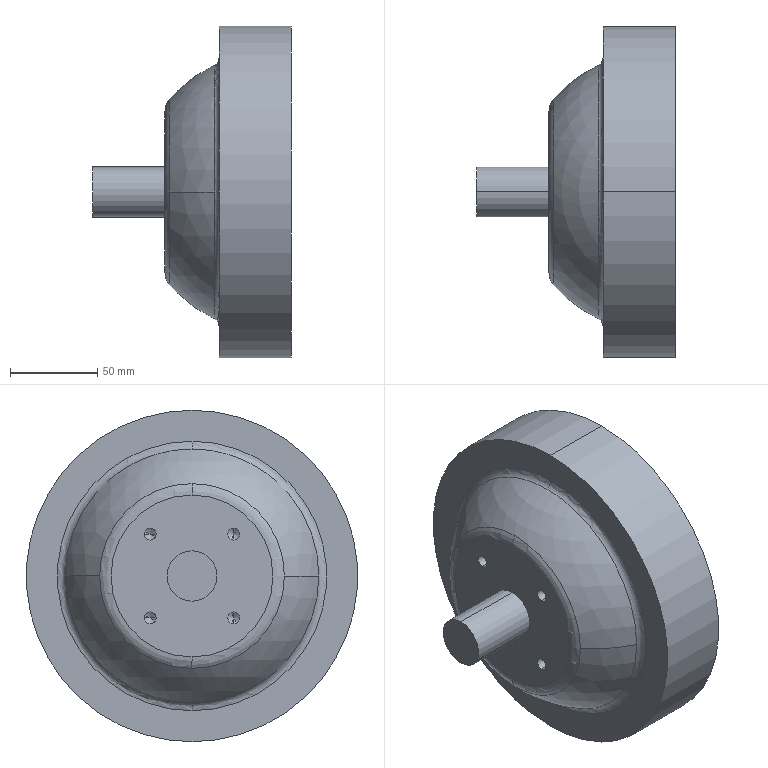Part | NX | features BREP 1 | 1 solid | 30 faces | box 114 x 190 x 190 mm | volume 1604284 mm3 | cylinder 12 | cone 8 | plane 4 | torus 4 | sphere 2 | commonest cylinder face diameters 6.8 x8 28.848 x2 190 x2
STEP:
#1=CARTESIAN_POINT('',(-72.5,0.,-46.402));
#2=VERTEX_POINT('',#1);
#3=CARTESIAN_POINT('',(-72.5,0.,46.402));
#4=VERTEX_POINT('',#3);
#5=CARTESIAN_POINT('',(-72.5,0.,0.));
#6=DIRECTION('',(-1.,0.,0.));
#7=DIRECTION('',(0.,0.,-1.));
#8=AXIS2_PLACEMENT_3D('',#5,#6,#7);
#9=CIRCLE('',#8,46.402);
#10=EDGE_CURVE('',#2,#4,#9,.T.);
#11=ORIENTED_EDGE('',*,*,#10,.T.);
#12=CARTESIAN_POINT('',(-72.5,0.,0.));
#13=DIRECTION('',(-1.,0.,0.));
#14=DIRECTION('',(0.,0.,1.));
#15=AXIS2_PLACEMENT_3D('',#12,#13,#14);
#16=CIRCLE('',#15,46.402);
#17=EDGE_CURVE('',#4,#2,#16,.T.);
#18=ORIENTED_EDGE('',*,*,#17,.T.);
#19=EDGE_LOOP('',(#11,#18));
#20=FACE_BOUND('',#19,.T.);
#21=CARTESIAN_POINT('',(-72.5,0.,14.424));
#22=VERTEX_POINT('',#21);
#23=CARTESIAN_POINT('',(-72.5,0.,-14.424));
#24=VERTEX_POINT('',#23);
#25=CARTESIAN_POINT('',(-72.5,0.,0.));
#26=DIRECTION('',(1.,0.,0.));
#27=DIRECTION('',(0.,0.,1.));
#28=AXIS2_PLACEMENT_3D('',#25,#26,#27);
#29=CIRCLE('',#28,14.424);
#30=EDGE_CURVE('',#22,#24,#29,.T.);
#31=ORIENTED_EDGE('',*,*,#30,.T.);
#32=CARTESIAN_POINT('',(-72.5,0.,0.));
#33=DIRECTION('',(1.,0.,0.));
#34=DIRECTION('',(0.,0.,-1.));
#35=AXIS2_PLACEMENT_3D('',#32,#33,#34);
#36=CIRCLE('',#35,14.424);
#37=EDGE_CURVE('',#24,#22,#36,.T.);
#38=ORIENTED_EDGE('',*,*,#37,.T.);
#39=EDGE_LOOP('',(#31,#38));
#40=FACE_BOUND('',#39,.T.);
#41=CARTESIAN_POINT('',(-72.5,24.,-27.4));
#42=VERTEX_POINT('',#41);
#43=CARTESIAN_POINT('',(-72.5,24.,-20.6));
#44=VERTEX_POINT('',#43);
#45=CARTESIAN_POINT('',(-72.5,24.,-24.));
#46=DIRECTION('',(1.,0.,0.));
#47=DIRECTION('',(0.,0.,-1.));
#48=AXIS2_PLACEMENT_3D('',#45,#46,#47);
#49=CIRCLE('',#48,3.4);
#50=EDGE_CURVE('',#42,#44,#49,.T.);
#51=ORIENTED_EDGE('',*,*,#50,.T.);
#52=CARTESIAN_POINT('',(-72.5,24.,-24.));
#53=DIRECTION('',(1.,0.,0.));
#54=DIRECTION('',(0.,0.,1.));
#55=AXIS2_PLACEMENT_3D('',#52,#53,#54);
#56=CIRCLE('',#55,3.4);
#57=EDGE_CURVE('',#44,#42,#56,.T.);
#58=ORIENTED_EDGE('',*,*,#57,.T.);
#59=EDGE_LOOP('',(#51,#58));
#60=FACE_BOUND('',#59,.T.);
#61=CARTESIAN_POINT('',(-72.5,24.,20.6));
#62=VERTEX_POINT('',#61);
#63=CARTESIAN_POINT('',(-72.5,24.,27.4));
#64=VERTEX_POINT('',#63);
#65=CARTESIAN_POINT('',(-72.5,24.,24.));
#66=DIRECTION('',(1.,0.,0.));
#67=DIRECTION('',(0.,0.,-1.));
#68=AXIS2_PLACEMENT_3D('',#65,#66,#67);
#69=CIRCLE('',#68,3.4);
#70=EDGE_CURVE('',#62,#64,#69,.T.);
#71=ORIENTED_EDGE('',*,*,#70,.T.);
#72=CARTESIAN_POINT('',(-72.5,24.,24.));
#73=DIRECTION('',(1.,0.,0.));
#74=DIRECTION('',(0.,0.,1.));
#75=AXIS2_PLACEMENT_3D('',#72,#73,#74);
#76=CIRCLE('',#75,3.4);
#77=EDGE_CURVE('',#64,#62,#76,.T.);
#78=ORIENTED_EDGE('',*,*,#77,.T.);
#79=EDGE_LOOP('',(#71,#78));
#80=FACE_BOUND('',#79,.T.);
#81=CARTESIAN_POINT('',(-72.5,-24.,20.6));
#82=VERTEX_POINT('',#81);
#83=CARTESIAN_POINT('',(-72.5,-24.,27.4));
#84=VERTEX_POINT('',#83);
#85=CARTESIAN_POINT('',(-72.5,-24.,24.));
#86=DIRECTION('',(1.,0.,0.));
#87=DIRECTION('',(0.,0.,-1.));
#88=AXIS2_PLACEMENT_3D('',#85,#86,#87);
#89=CIRCLE('',#88,3.4);
#90=EDGE_CURVE('',#82,#84,#89,.T.);
#91=ORIENTED_EDGE('',*,*,#90,.T.);
#92=CARTESIAN_POINT('',(-72.5,-24.,24.));
#93=DIRECTION('',(1.,0.,0.));
#94=DIRECTION('',(0.,0.,1.));
#95=AXIS2_PLACEMENT_3D('',#92,#93,#94);
#96=CIRCLE('',#95,3.4);
#97=EDGE_CURVE('',#84,#82,#96,.T.);
#98=ORIENTED_EDGE('',*,*,#97,.T.);
#99=EDGE_LOOP('',(#91,#98));
#100=FACE_BOUND('',#99,.T.);
#101=CARTESIAN_POINT('',(-72.5,-24.,-27.4));
#102=VERTEX_POINT('',#101);
#103=CARTESIAN_POINT('',(-72.5,-24.,-20.6));
#104=VERTEX_POINT('',#103);
#105=CARTESIAN_POINT('',(-72.5,-24.,-24.));
#106=DIRECTION('',(1.,0.,0.));
#107=DIRECTION('',(0.,0.,-1.));
#108=AXIS2_PLACEMENT_3D('',#105,#106,#107);
#109=CIRCLE('',#108,3.4);
#110=EDGE_CURVE('',#102,#104,#109,.T.);
#111=ORIENTED_EDGE('',*,*,#110,.T.);
#112=CARTESIAN_POINT('',(-72.5,-24.,-24.));
#113=DIRECTION('',(1.,0.,0.));
#114=DIRECTION('',(0.,0.,1.));
#115=AXIS2_PLACEMENT_3D('',#112,#113,#114);
#116=CIRCLE('',#115,3.4);
#117=EDGE_CURVE('',#104,#102,#116,.T.);
#118=ORIENTED_EDGE('',*,*,#117,.T.);
#119=EDGE_LOOP('',(#111,#118));
#120=FACE_BOUND('',#119,.T.);
#121=CARTESIAN_POINT('',(-72.5,-48.837,-48.837));
#122=DIRECTION('',(-1.,0.,0.));
#123=DIRECTION('',(0.,0.,1.));
#124=AXIS2_PLACEMENT_3D('',#121,#122,#123);
#125=PLANE('',#124);
#126=ADVANCED_FACE('',(#20,#40,#60,#80,#100,#120),#125,.T.);
#127=CARTESIAN_POINT('',(-70.048,0.,-52.961));
#128=VERTEX_POINT('',#127);
#129=CARTESIAN_POINT('',(-70.048,52.961,0.));
#130=VERTEX_POINT('',#129);
#131=CARTESIAN_POINT('',(-70.048,0.,0.));
#132=DIRECTION('',(1.,0.,0.));
#133=DIRECTION('',(0.,0.,-1.));
#134=AXIS2_PLACEMENT_3D('',#131,#132,#133);
#135=CIRCLE('',#134,52.961);
#136=EDGE_CURVE('',#128,#130,#135,.T.);
#137=ORIENTED_EDGE('',*,*,#136,.F.);
#138=CARTESIAN_POINT('',(-62.5,0.,-46.402));
#139=DIRECTION('',(0.,-1.,0.));
#140=DIRECTION('',(-1.,0.,0.));
#141=AXIS2_PLACEMENT_3D('',#138,#139,#140);
#142=CIRCLE('',#141,10.);
#143=EDGE_CURVE('',#2,#128,#142,.T.);
#144=ORIENTED_EDGE('',*,*,#143,.F.);
#145=ORIENTED_EDGE('',*,*,#17,.F.);
#146=CARTESIAN_POINT('',(-70.048,0.,52.961));
#147=VERTEX_POINT('',#146);
#148=CARTESIAN_POINT('',(-62.5,0.,46.402));
#149=DIRECTION('',(0.,1.,0.));
#150=DIRECTION('',(-1.,0.,0.));
#151=AXIS2_PLACEMENT_3D('',#148,#149,#150);
#152=CIRCLE('',#151,10.);
#153=EDGE_CURVE('',#4,#147,#152,.T.);
#154=ORIENTED_EDGE('',*,*,#153,.T.);
#155=CARTESIAN_POINT('',(-70.048,0.,0.));
#156=DIRECTION('',(1.,0.,0.));
#157=DIRECTION('',(0.,1.,0.));
#158=AXIS2_PLACEMENT_3D('',#155,#156,#157);
#159=CIRCLE('',#158,52.961);
#160=EDGE_CURVE('',#130,#147,#159,.T.);
#161=ORIENTED_EDGE('',*,*,#160,.F.);
#162=EDGE_LOOP('',(#137,#144,#145,#154,#161));
#163=FACE_BOUND('',#162,.T.);
#164=CARTESIAN_POINT('',(-62.5,0.,0.));
#165=DIRECTION('',(-1.,0.,0.));
#166=DIRECTION('',(0.,0.,1.));
#167=AXIS2_PLACEMENT_3D('',#164,#165,#166);
#168=TOROIDAL_SURFACE('',#167,46.402,10.);
#169=ADVANCED_FACE('',(#163),#168,.T.);
#170=CARTESIAN_POINT('',(-44.225,-72.702,0.));
#171=VERTEX_POINT('',#170);
#172=CARTESIAN_POINT('',(-70.048,-52.961,0.));
#173=VERTEX_POINT('',#172);
#174=CARTESIAN_POINT('',(-9.104,0.,0.));
#175=DIRECTION('',(0.,0.,-1.));
#176=DIRECTION('',(-0.435,-0.9004,0.));
#177=AXIS2_PLACEMENT_3D('',#174,#175,#176);
#178=CIRCLE('',#177,80.74);
#179=EDGE_CURVE('',#171,#173,#178,.T.);
#180=ORIENTED_EDGE('',*,*,#179,.F.);
#181=CARTESIAN_POINT('',(-44.225,0.,72.702));
#182=VERTEX_POINT('',#181);
#183=CARTESIAN_POINT('',(-44.225,0.,0.));
#184=DIRECTION('',(-1.,0.,0.));
#185=DIRECTION('',(0.,-1.,0.));
#186=AXIS2_PLACEMENT_3D('',#183,#184,#185);
#187=CIRCLE('',#186,72.702);
#188=EDGE_CURVE('',#171,#182,#187,.T.);
#189=ORIENTED_EDGE('',*,*,#188,.T.);
#190=CARTESIAN_POINT('',(-44.225,72.702,0.));
#191=VERTEX_POINT('',#190);
#192=CARTESIAN_POINT('',(-44.225,0.,0.));
#193=DIRECTION('',(-1.,0.,0.));
#194=DIRECTION('',(0.,0.,1.));
#195=AXIS2_PLACEMENT_3D('',#192,#193,#194);
#196=CIRCLE('',#195,72.702);
#197=EDGE_CURVE('',#182,#191,#196,.T.);
#198=ORIENTED_EDGE('',*,*,#197,.T.);
#199=CARTESIAN_POINT('',(-9.104,0.,0.));
#200=DIRECTION('',(0.,0.,1.));
#201=DIRECTION('',(-0.435,0.9004,0.));
#202=AXIS2_PLACEMENT_3D('',#199,#200,#201);
#203=CIRCLE('',#202,80.74);
#204=EDGE_CURVE('',#191,#130,#203,.T.);
#205=ORIENTED_EDGE('',*,*,#204,.T.);
#206=ORIENTED_EDGE('',*,*,#160,.T.);
#207=CARTESIAN_POINT('',(-70.048,0.,0.));
#208=DIRECTION('',(1.,0.,0.));
#209=DIRECTION('',(0.,0.,1.));
#210=AXIS2_PLACEMENT_3D('',#207,#208,#209);
#211=CIRCLE('',#210,52.961);
#212=EDGE_CURVE('',#147,#173,#211,.T.);
#213=ORIENTED_EDGE('',*,*,#212,.T.);
#214=EDGE_LOOP('',(#180,#189,#198,#205,#206,#213));
#215=FACE_BOUND('',#214,.T.);
#216=CARTESIAN_POINT('',(-9.104,0.,0.));
#217=DIRECTION('',(0.,0.,1.));
#218=DIRECTION('',(0.,1.,0.));
#219=AXIS2_PLACEMENT_3D('',#216,#217,#218);
#220=SPHERICAL_SURFACE('',#219,80.74);
#221=ADVANCED_FACE('',(#215),#220,.T.);
#222=CARTESIAN_POINT('',(-70.048,0.,0.));
#223=DIRECTION('',(1.,0.,0.));
#224=DIRECTION('',(0.,-1.,0.));
#225=AXIS2_PLACEMENT_3D('',#222,#223,#224);
#226=CIRCLE('',#225,52.961);
#227=EDGE_CURVE('',#173,#128,#226,.T.);
#228=ORIENTED_EDGE('',*,*,#227,.F.);
#229=ORIENTED_EDGE('',*,*,#212,.F.);
#230=ORIENTED_EDGE('',*,*,#153,.F.);
#231=ORIENTED_EDGE('',*,*,#10,.F.);
#232=ORIENTED_EDGE('',*,*,#143,.T.);
#233=EDGE_LOOP('',(#228,#229,#230,#231,#232));
#234=FACE_BOUND('',#233,.T.);
#235=CARTESIAN_POINT('',(-62.5,0.,0.));
#236=DIRECTION('',(-1.,0.,0.));
#237=DIRECTION('',(0.,0.,-1.));
#238=AXIS2_PLACEMENT_3D('',#235,#236,#237);
#239=TOROIDAL_SURFACE('',#238,46.402,10.);
#240=ADVANCED_FACE('',(#234),#239,.T.);
#241=ORIENTED_EDGE('',*,*,#227,.T.);
#242=ORIENTED_EDGE('',*,*,#136,.T.);
#243=ORIENTED_EDGE('',*,*,#204,.F.);
#244=CARTESIAN_POINT('',(-44.225,0.,-72.702));
#245=VERTEX_POINT('',#244);
#246=CARTESIAN_POINT('',(-44.225,0.,0.));
#247=DIRECTION('',(-1.,0.,0.));
#248=DIRECTION('',(0.,1.,0.));
#249=AXIS2_PLACEMENT_3D('',#246,#247,#248);
#250=CIRCLE('',#249,72.702);
#251=EDGE_CURVE('',#191,#245,#250,.T.);
#252=ORIENTED_EDGE('',*,*,#251,.T.);
#253=CARTESIAN_POINT('',(-44.225,0.,0.));
#254=DIRECTION('',(-1.,0.,0.));
#255=DIRECTION('',(0.,0.,-1.));
#256=AXIS2_PLACEMENT_3D('',#253,#254,#255);
#257=CIRCLE('',#256,72.702);
#258=EDGE_CURVE('',#245,#171,#257,.T.);
#259=ORIENTED_EDGE('',*,*,#258,.T.);
#260=ORIENTED_EDGE('',*,*,#179,.T.);
#261=EDGE_LOOP('',(#241,#242,#243,#252,#259,#260));
#262=FACE_BOUND('',#261,.T.);
#263=CARTESIAN_POINT('',(-9.104,0.,0.));
#264=DIRECTION('',(0.,0.,-1.));
#265=DIRECTION('',(0.,-1.,0.));
#266=AXIS2_PLACEMENT_3D('',#263,#264,#265);
#267=SPHERICAL_SURFACE('',#266,80.74);
#268=ADVANCED_FACE('',(#262),#267,.T.);
#269=CARTESIAN_POINT('',(-41.4,0.,-77.204));
#270=VERTEX_POINT('',#269);
#271=CARTESIAN_POINT('',(-46.4,0.,-77.204));
#272=DIRECTION('',(0.,-1.,0.));
#273=DIRECTION('',(1.,0.,0.));
#274=AXIS2_PLACEMENT_3D('',#271,#272,#273);
#275=CIRCLE('',#274,5.);
#276=EDGE_CURVE('',#270,#245,#275,.T.);
#277=ORIENTED_EDGE('',*,*,#276,.F.);
#278=CARTESIAN_POINT('',(-41.4,0.,77.204));
#279=VERTEX_POINT('',#278);
#280=CARTESIAN_POINT('',(-41.4,0.,0.));
#281=DIRECTION('',(1.,0.,0.));
#282=DIRECTION('',(0.,0.,1.));
#283=AXIS2_PLACEMENT_3D('',#280,#281,#282);
#284=CIRCLE('',#283,77.204);
#285=EDGE_CURVE('',#279,#270,#284,.T.);
#286=ORIENTED_EDGE('',*,*,#285,.F.);
#287=CARTESIAN_POINT('',(-46.4,0.,77.204));
#288=DIRECTION('',(0.,1.,0.));
#289=DIRECTION('',(1.,0.,0.));
#290=AXIS2_PLACEMENT_3D('',#287,#288,#289);
#291=CIRCLE('',#290,5.);
#292=EDGE_CURVE('',#279,#182,#291,.T.);
#293=ORIENTED_EDGE('',*,*,#292,.T.);
#294=ORIENTED_EDGE('',*,*,#188,.F.);
#295=ORIENTED_EDGE('',*,*,#258,.F.);
#296=EDGE_LOOP('',(#277,#286,#293,#294,#295));
#297=FACE_BOUND('',#296,.T.);
#298=CARTESIAN_POINT('',(-46.4,0.,0.));
#299=DIRECTION('',(1.,0.,0.));
#300=DIRECTION('',(0.,0.,-1.));
#301=AXIS2_PLACEMENT_3D('',#298,#299,#300);
#302=TOROIDAL_SURFACE('',#301,77.204,5.);
#303=ADVANCED_FACE('',(#297),#302,.F.);
#304=ORIENTED_EDGE('',*,*,#251,.F.);
#305=ORIENTED_EDGE('',*,*,#197,.F.);
#306=ORIENTED_EDGE('',*,*,#292,.F.);
#307=CARTESIAN_POINT('',(-41.4,0.,0.));
#308=DIRECTION('',(1.,0.,0.));
#309=DIRECTION('',(0.,0.,-1.));
#310=AXIS2_PLACEMENT_3D('',#307,#308,#309);
#311=CIRCLE('',#310,77.204);
#312=EDGE_CURVE('',#270,#279,#311,.T.);
#313=ORIENTED_EDGE('',*,*,#312,.F.);
#314=ORIENTED_EDGE('',*,*,#276,.T.);
#315=EDGE_LOOP('',(#304,#305,#306,#313,#314));
#316=FACE_BOUND('',#315,.T.);
#317=CARTESIAN_POINT('',(-46.4,0.,0.));
#318=DIRECTION('',(1.,0.,0.));
#319=DIRECTION('',(0.,0.,1.));
#320=AXIS2_PLACEMENT_3D('',#317,#318,#319);
#321=TOROIDAL_SURFACE('',#320,77.204,5.);
#322=ADVANCED_FACE('',(#316),#321,.F.);
#323=CARTESIAN_POINT('',(-41.4,0.,95.));
#324=VERTEX_POINT('',#323);
#325=CARTESIAN_POINT('',(-41.4,0.,-95.));
#326=VERTEX_POINT('',#325);
#327=CARTESIAN_POINT('',(-41.4,0.,0.));
#328=DIRECTION('',(-1.,0.,0.));
#329=DIRECTION('',(0.,0.,1.));
#330=AXIS2_PLACEMENT_3D('',#327,#328,#329);
#331=CIRCLE('',#330,95.);
#332=EDGE_CURVE('',#324,#326,#331,.T.);
#333=ORIENTED_EDGE('',*,*,#332,.T.);
#334=CARTESIAN_POINT('',(-41.4,0.,0.));
#335=DIRECTION('',(-1.,0.,0.));
#336=DIRECTION('',(0.,0.,-1.));
#337=AXIS2_PLACEMENT_3D('',#334,#335,#336);
#338=CIRCLE('',#337,95.);
#339=EDGE_CURVE('',#326,#324,#338,.T.);
#340=ORIENTED_EDGE('',*,*,#339,.T.);
#341=EDGE_LOOP('',(#333,#340));
#342=FACE_BOUND('',#341,.T.);
#343=ORIENTED_EDGE('',*,*,#312,.T.);
#344=ORIENTED_EDGE('',*,*,#285,.T.);
#345=EDGE_LOOP('',(#343,#344));
#346=FACE_BOUND('',#345,.T.);
#347=CARTESIAN_POINT('',(-41.4,-98.933,-98.933));
#348=DIRECTION('',(-1.,0.,0.));
#349=DIRECTION('',(0.,0.,1.));
#350=AXIS2_PLACEMENT_3D('',#347,#348,#349);
#351=PLANE('',#350);
#352=ADVANCED_FACE('',(#342,#346),#351,.T.);
#353=ORIENTED_EDGE('',*,*,#339,.F.);
#354=CARTESIAN_POINT('',(0.,0.,-95.));
#355=VERTEX_POINT('',#354);
#356=CARTESIAN_POINT('',(0.,0.,-95.));
#357=DIRECTION('',(-1.,0.,0.));
#358=VECTOR('',#357,1000.);
#359=LINE('',#356,#358);
#360=EDGE_CURVE('',#355,#326,#359,.T.);
#361=ORIENTED_EDGE('',*,*,#360,.F.);
#362=CARTESIAN_POINT('',(0.,0.,95.));
#363=VERTEX_POINT('',#362);
#364=CARTESIAN_POINT('',(0.,0.,0.));
#365=DIRECTION('',(1.,0.,0.));
#366=DIRECTION('',(0.,0.,1.));
#367=AXIS2_PLACEMENT_3D('',#364,#365,#366);
#368=CIRCLE('',#367,95.);
#369=EDGE_CURVE('',#363,#355,#368,.T.);
#370=ORIENTED_EDGE('',*,*,#369,.F.);
#371=CARTESIAN_POINT('',(0.,0.,95.));
#372=DIRECTION('',(-1.,0.,0.));
#373=VECTOR('',#372,1000.);
#374=LINE('',#371,#373);
#375=EDGE_CURVE('',#363,#324,#374,.T.);
#376=ORIENTED_EDGE('',*,*,#375,.T.);
#377=EDGE_LOOP('',(#353,#361,#370,#376));
#378=FACE_BOUND('',#377,.T.);
#379=CARTESIAN_POINT('',(-30.4,0.,0.));
#380=DIRECTION('',(1.,0.,0.));
#381=DIRECTION('',(0.,0.,-1.));
#382=AXIS2_PLACEMENT_3D('',#379,#380,#381);
#383=CYLINDRICAL_SURFACE('',#382,95.);
#384=ADVANCED_FACE('',(#378),#383,.T.);
#385=ORIENTED_EDGE('',*,*,#375,.F.);
#386=CARTESIAN_POINT('',(0.,0.,0.));
#387=DIRECTION('',(1.,0.,0.));
#388=DIRECTION('',(0.,0.,-1.));
#389=AXIS2_PLACEMENT_3D('',#386,#387,#388);
#390=CIRCLE('',#389,95.);
#391=EDGE_CURVE('',#355,#363,#390,.T.);
#392=ORIENTED_EDGE('',*,*,#391,.F.);
#393=ORIENTED_EDGE('',*,*,#360,.T.);
#394=ORIENTED_EDGE('',*,*,#332,.F.);
#395=EDGE_LOOP('',(#385,#392,#393,#394));
#396=FACE_BOUND('',#395,.T.);
#397=CARTESIAN_POINT('',(-30.4,0.,0.));
#398=DIRECTION('',(1.,0.,0.));
#399=DIRECTION('',(0.,0.,-1.));
#400=AXIS2_PLACEMENT_3D('',#397,#398,#399);
#401=CYLINDRICAL_SURFACE('',#400,95.);
#402=ADVANCED_FACE('',(#396),#401,.T.);
#403=ORIENTED_EDGE('',*,*,#391,.T.);
#404=ORIENTED_EDGE('',*,*,#369,.T.);
#405=EDGE_LOOP('',(#403,#404));
#406=FACE_BOUND('',#405,.T.);
#407=CARTESIAN_POINT('',(0.,-98.933,98.933));
#408=DIRECTION('',(1.,0.,0.));
#409=DIRECTION('',(0.,1.,0.));
#410=AXIS2_PLACEMENT_3D('',#407,#408,#409);
#411=PLANE('',#410);
#412=ADVANCED_FACE('',(#406),#411,.T.);
#413=CARTESIAN_POINT('',(-114.,0.,-14.424));
#414=VERTEX_POINT('',#413);
#415=CARTESIAN_POINT('',(-114.,0.,-14.424));
#416=DIRECTION('',(1.,0.,0.));
#417=VECTOR('',#416,1000.);
#418=LINE('',#415,#417);
#419=EDGE_CURVE('',#414,#24,#418,.T.);
#420=ORIENTED_EDGE('',*,*,#419,.F.);
#421=CARTESIAN_POINT('',(-114.,0.,14.424));
#422=VERTEX_POINT('',#421);
#423=CARTESIAN_POINT('',(-114.,0.,0.));
#424=DIRECTION('',(-1.,0.,0.));
#425=DIRECTION('',(0.,0.,1.));
#426=AXIS2_PLACEMENT_3D('',#423,#424,#425);
#427=CIRCLE('',#426,14.424);
#428=EDGE_CURVE('',#422,#414,#427,.T.);
#429=ORIENTED_EDGE('',*,*,#428,.F.);
#430=CARTESIAN_POINT('',(-114.,0.,14.424));
#431=DIRECTION('',(1.,0.,0.));
#432=VECTOR('',#431,1000.);
#433=LINE('',#430,#432);
#434=EDGE_CURVE('',#422,#22,#433,.T.);
#435=ORIENTED_EDGE('',*,*,#434,.T.);
#436=ORIENTED_EDGE('',*,*,#37,.F.);
#437=EDGE_LOOP('',(#420,#429,#435,#436));
#438=FACE_BOUND('',#437,.T.);
#439=CARTESIAN_POINT('',(22.798,0.,0.));
#440=DIRECTION('',(-1.,0.,0.));
#441=DIRECTION('',(0.,0.,1.));
#442=AXIS2_PLACEMENT_3D('',#439,#440,#441);
#443=CYLINDRICAL_SURFACE('',#442,14.424);
#444=ADVANCED_FACE('',(#438),#443,.T.);
#445=ORIENTED_EDGE('',*,*,#30,.F.);
#446=ORIENTED_EDGE('',*,*,#434,.F.);
#447=CARTESIAN_POINT('',(-114.,0.,0.));
#448=DIRECTION('',(-1.,0.,0.));
#449=DIRECTION('',(0.,0.,-1.));
#450=AXIS2_PLACEMENT_3D('',#447,#448,#449);
#451=CIRCLE('',#450,14.424);
#452=EDGE_CURVE('',#414,#422,#451,.T.);
#453=ORIENTED_EDGE('',*,*,#452,.F.);
#454=ORIENTED_EDGE('',*,*,#419,.T.);
#455=EDGE_LOOP('',(#445,#446,#453,#454));
#456=FACE_BOUND('',#455,.T.);
#457=CARTESIAN_POINT('',(22.798,0.,0.));
#458=DIRECTION('',(-1.,0.,0.));
#459=DIRECTION('',(0.,0.,1.));
#460=AXIS2_PLACEMENT_3D('',#457,#458,#459);
#461=CYLINDRICAL_SURFACE('',#460,14.424);
#462=ADVANCED_FACE('',(#456),#461,.T.);
#463=ORIENTED_EDGE('',*,*,#452,.T.);
#464=ORIENTED_EDGE('',*,*,#428,.T.);
#465=EDGE_LOOP('',(#463,#464));
#466=FACE_BOUND('',#465,.T.);
#467=CARTESIAN_POINT('',(-114.,-10.525,-10.525));
#468=DIRECTION('',(-1.,0.,0.));
#469=DIRECTION('',(0.,0.,1.));
#470=AXIS2_PLACEMENT_3D('',#467,#468,#469);
#471=PLANE('',#470);
#472=ADVANCED_FACE('',(#466),#471,.T.);
#473=CARTESIAN_POINT('',(-56.75,24.,-27.4));
#474=VERTEX_POINT('',#473);
#475=CARTESIAN_POINT('',(-72.5,24.,-27.4));
#476=DIRECTION('',(1.,0.,0.));
#477=VECTOR('',#476,1000.);
#478=LINE('',#475,#477);
#479=EDGE_CURVE('',#42,#474,#478,.T.);
#480=ORIENTED_EDGE('',*,*,#479,.F.);
#481=ORIENTED_EDGE('',*,*,#57,.F.);
#482=CARTESIAN_POINT('',(-56.75,24.,-20.6));
#483=VERTEX_POINT('',#482);
#484=CARTESIAN_POINT('',(-72.5,24.,-20.6));
#485=DIRECTION('',(1.,0.,0.));
#486=VECTOR('',#485,1000.);
#487=LINE('',#484,#486);
#488=EDGE_CURVE('',#44,#483,#487,.T.);
#489=ORIENTED_EDGE('',*,*,#488,.T.);
#490=CARTESIAN_POINT('',(-56.75,20.6,-24.));
#491=VERTEX_POINT('',#490);
#492=CARTESIAN_POINT('',(-56.75,24.,-24.));
#493=DIRECTION('',(-1.,0.,0.));
#494=DIRECTION('',(0.,-1.,0.));
#495=AXIS2_PLACEMENT_3D('',#492,#493,#494);
#496=CIRCLE('',#495,3.4);
#497=EDGE_CURVE('',#491,#483,#496,.T.);
#498=ORIENTED_EDGE('',*,*,#497,.F.);
#499=CARTESIAN_POINT('',(-56.75,24.,-24.));
#500=DIRECTION('',(-1.,0.,0.));
#501=DIRECTION('',(0.,0.,-1.));
#502=AXIS2_PLACEMENT_3D('',#499,#500,#501);
#503=CIRCLE('',#502,3.4);
#504=EDGE_CURVE('',#474,#491,#503,.T.);
#505=ORIENTED_EDGE('',*,*,#504,.F.);
#506=EDGE_LOOP('',(#480,#481,#489,#498,#505));
#507=FACE_BOUND('',#506,.T.);
#508=CARTESIAN_POINT('',(-56.75,24.,-24.));
#509=DIRECTION('',(-1.,0.,0.));
#510=DIRECTION('',(0.,0.,1.));
#511=AXIS2_PLACEMENT_3D('',#508,#509,#510);
#512=CYLINDRICAL_SURFACE('',#511,3.4);
#513=ADVANCED_FACE('',(#507),#512,.F.);
#514=CARTESIAN_POINT('',(-54.707,24.,-24.));
#515=VERTEX_POINT('',#514);
#516=CARTESIAN_POINT('',(-56.75,27.4,-24.));
#517=VERTEX_POINT('',#516);
#518=CARTESIAN_POINT('',(-56.75,27.4,-24.));
#519=DIRECTION('',(0.515,-0.8572,0.));
#520=VECTOR('',#519,1000.);
#521=LINE('',#518,#520);
#522=EDGE_CURVE('',#515,#517,#521,.F.);
#523=ORIENTED_EDGE('',*,*,#522,.T.);
#524=CARTESIAN_POINT('',(-56.75,24.,-24.));
#525=DIRECTION('',(-1.,0.,0.));
#526=DIRECTION('',(0.,1.,0.));
#527=AXIS2_PLACEMENT_3D('',#524,#525,#526);
#528=CIRCLE('',#527,3.4);
#529=EDGE_CURVE('',#517,#474,#528,.T.);
#530=ORIENTED_EDGE('',*,*,#529,.T.);
#531=ORIENTED_EDGE('',*,*,#504,.T.);
#532=CARTESIAN_POINT('',(-56.75,20.6,-24.));
#533=DIRECTION('',(0.515,0.8572,0.));
#534=VECTOR('',#533,1000.);
#535=LINE('',#532,#534);
#536=EDGE_CURVE('',#515,#491,#535,.F.);
#537=ORIENTED_EDGE('',*,*,#536,.F.);
#538=EDGE_LOOP('',(#523,#530,#531,#537));
#539=FACE_BOUND('',#538,.T.);
#540=CARTESIAN_POINT('',(-55.819,24.,-24.));
#541=DIRECTION('',(-1.,0.,0.));
#542=DIRECTION('',(0.,-1.,0.));
#543=AXIS2_PLACEMENT_3D('',#540,#541,#542);
#544=CONICAL_SURFACE('',#543,1.85,1.03);
#545=ADVANCED_FACE('',(#539),#544,.F.);
#546=ORIENTED_EDGE('',*,*,#536,.T.);
#547=ORIENTED_EDGE('',*,*,#497,.T.);
#548=CARTESIAN_POINT('',(-56.75,24.,-24.));
#549=DIRECTION('',(-1.,0.,0.));
#550=DIRECTION('',(0.,0.,1.));
#551=AXIS2_PLACEMENT_3D('',#548,#549,#550);
#552=CIRCLE('',#551,3.4);
#553=EDGE_CURVE('',#483,#517,#552,.T.);
#554=ORIENTED_EDGE('',*,*,#553,.T.);
#555=ORIENTED_EDGE('',*,*,#522,.F.);
#556=EDGE_LOOP('',(#546,#547,#554,#555));
#557=FACE_BOUND('',#556,.T.);
#558=CARTESIAN_POINT('',(-55.819,24.,-24.));
#559=DIRECTION('',(-1.,0.,0.));
#560=DIRECTION('',(0.,-1.,0.));
#561=AXIS2_PLACEMENT_3D('',#558,#559,#560);
#562=CONICAL_SURFACE('',#561,1.85,1.03);
#563=ADVANCED_FACE('',(#557),#562,.F.);
#564=ORIENTED_EDGE('',*,*,#529,.F.);
#565=ORIENTED_EDGE('',*,*,#553,.F.);
#566=ORIENTED_EDGE('',*,*,#488,.F.);
#567=ORIENTED_EDGE('',*,*,#50,.F.);
#568=ORIENTED_EDGE('',*,*,#479,.T.);
#569=EDGE_LOOP('',(#564,#565,#566,#567,#568));
#570=FACE_BOUND('',#569,.T.);
#571=CARTESIAN_POINT('',(-56.75,24.,-24.));
#572=DIRECTION('',(-1.,0.,0.));
#573=DIRECTION('',(0.,0.,1.));
#574=AXIS2_PLACEMENT_3D('',#571,#572,#573);
#575=CYLINDRICAL_SURFACE('',#574,3.4);
#576=ADVANCED_FACE('',(#570),#575,.F.);
#577=CARTESIAN_POINT('',(-56.75,24.,20.6));
#578=VERTEX_POINT('',#577);
#579=CARTESIAN_POINT('',(-72.5,24.,20.6));
#580=DIRECTION('',(1.,0.,0.));
#581=VECTOR('',#580,1000.);
#582=LINE('',#579,#581);
#583=EDGE_CURVE('',#62,#578,#582,.T.);
#584=ORIENTED_EDGE('',*,*,#583,.F.);
#585=ORIENTED_EDGE('',*,*,#77,.F.);
#586=CARTESIAN_POINT('',(-56.75,24.,27.4));
#587=VERTEX_POINT('',#586);
#588=CARTESIAN_POINT('',(-72.5,24.,27.4));
#589=DIRECTION('',(1.,0.,0.));
#590=VECTOR('',#589,1000.);
#591=LINE('',#588,#590);
#592=EDGE_CURVE('',#64,#587,#591,.T.);
#593=ORIENTED_EDGE('',*,*,#592,.T.);
#594=CARTESIAN_POINT('',(-56.75,20.6,24.));
#595=VERTEX_POINT('',#594);
#596=CARTESIAN_POINT('',(-56.75,24.,24.));
#597=DIRECTION('',(-1.,0.,0.));
#598=DIRECTION('',(0.,-1.,0.));
#599=AXIS2_PLACEMENT_3D('',#596,#597,#598);
#600=CIRCLE('',#599,3.4);
#601=EDGE_CURVE('',#595,#587,#600,.T.);
#602=ORIENTED_EDGE('',*,*,#601,.F.);
#603=CARTESIAN_POINT('',(-56.75,24.,24.));
#604=DIRECTION('',(-1.,0.,0.));
#605=DIRECTION('',(0.,0.,-1.));
#606=AXIS2_PLACEMENT_3D('',#603,#604,#605);
#607=CIRCLE('',#606,3.4);
#608=EDGE_CURVE('',#578,#595,#607,.T.);
#609=ORIENTED_EDGE('',*,*,#608,.F.);
#610=EDGE_LOOP('',(#584,#585,#593,#602,#609));
#611=FACE_BOUND('',#610,.T.);
#612=CARTESIAN_POINT('',(-56.75,24.,24.));
#613=DIRECTION('',(-1.,0.,0.));
#614=DIRECTION('',(0.,0.,1.));
#615=AXIS2_PLACEMENT_3D('',#612,#613,#614);
#616=CYLINDRICAL_SURFACE('',#615,3.4);
#617=ADVANCED_FACE('',(#611),#616,.F.);
#618=CARTESIAN_POINT('',(-54.707,24.,24.));
#619=VERTEX_POINT('',#618);
#620=CARTESIAN_POINT('',(-56.75,27.4,24.));
#621=VERTEX_POINT('',#620);
#622=CARTESIAN_POINT('',(-56.75,27.4,24.));
#623=DIRECTION('',(0.515,-0.8572,0.));
#624=VECTOR('',#623,1000.);
#625=LINE('',#622,#624);
#626=EDGE_CURVE('',#619,#621,#625,.F.);
#627=ORIENTED_EDGE('',*,*,#626,.T.);
#628=CARTESIAN_POINT('',(-56.75,24.,24.));
#629=DIRECTION('',(-1.,0.,0.));
#630=DIRECTION('',(0.,1.,0.));
#631=AXIS2_PLACEMENT_3D('',#628,#629,#630);
#632=CIRCLE('',#631,3.4);
#633=EDGE_CURVE('',#621,#578,#632,.T.);
#634=ORIENTED_EDGE('',*,*,#633,.T.);
#635=ORIENTED_EDGE('',*,*,#608,.T.);
#636=CARTESIAN_POINT('',(-56.75,20.6,24.));
#637=DIRECTION('',(0.515,0.8572,0.));
#638=VECTOR('',#637,1000.);
#639=LINE('',#636,#638);
#640=EDGE_CURVE('',#619,#595,#639,.F.);
#641=ORIENTED_EDGE('',*,*,#640,.F.);
#642=EDGE_LOOP('',(#627,#634,#635,#641));
#643=FACE_BOUND('',#642,.T.);
#644=CARTESIAN_POINT('',(-55.819,24.,24.));
#645=DIRECTION('',(-1.,0.,0.));
#646=DIRECTION('',(0.,-1.,0.));
#647=AXIS2_PLACEMENT_3D('',#644,#645,#646);
#648=CONICAL_SURFACE('',#647,1.85,1.03);
#649=ADVANCED_FACE('',(#643),#648,.F.);
#650=ORIENTED_EDGE('',*,*,#640,.T.);
#651=ORIENTED_EDGE('',*,*,#601,.T.);
#652=CARTESIAN_POINT('',(-56.75,24.,24.));
#653=DIRECTION('',(-1.,0.,0.));
#654=DIRECTION('',(0.,0.,1.));
#655=AXIS2_PLACEMENT_3D('',#652,#653,#654);
#656=CIRCLE('',#655,3.4);
#657=EDGE_CURVE('',#587,#621,#656,.T.);
#658=ORIENTED_EDGE('',*,*,#657,.T.);
#659=ORIENTED_EDGE('',*,*,#626,.F.);
#660=EDGE_LOOP('',(#650,#651,#658,#659));
#661=FACE_BOUND('',#660,.T.);
#662=CARTESIAN_POINT('',(-55.819,24.,24.));
#663=DIRECTION('',(-1.,0.,0.));
#664=DIRECTION('',(0.,-1.,0.));
#665=AXIS2_PLACEMENT_3D('',#662,#663,#664);
#666=CONICAL_SURFACE('',#665,1.85,1.03);
#667=ADVANCED_FACE('',(#661),#666,.F.);
#668=ORIENTED_EDGE('',*,*,#633,.F.);
#669=ORIENTED_EDGE('',*,*,#657,.F.);
#670=ORIENTED_EDGE('',*,*,#592,.F.);
#671=ORIENTED_EDGE('',*,*,#70,.F.);
#672=ORIENTED_EDGE('',*,*,#583,.T.);
#673=EDGE_LOOP('',(#668,#669,#670,#671,#672));
#674=FACE_BOUND('',#673,.T.);
#675=CARTESIAN_POINT('',(-56.75,24.,24.));
#676=DIRECTION('',(-1.,0.,0.));
#677=DIRECTION('',(0.,0.,1.));
#678=AXIS2_PLACEMENT_3D('',#675,#676,#677);
#679=CYLINDRICAL_SURFACE('',#678,3.4);
#680=ADVANCED_FACE('',(#674),#679,.F.);
#681=CARTESIAN_POINT('',(-56.75,-24.,20.6));
#682=VERTEX_POINT('',#681);
#683=CARTESIAN_POINT('',(-72.5,-24.,20.6));
#684=DIRECTION('',(1.,0.,0.));
#685=VECTOR('',#684,1000.);
#686=LINE('',#683,#685);
#687=EDGE_CURVE('',#82,#682,#686,.T.);
#688=ORIENTED_EDGE('',*,*,#687,.F.);
#689=ORIENTED_EDGE('',*,*,#97,.F.);
#690=CARTESIAN_POINT('',(-56.75,-24.,27.4));
#691=VERTEX_POINT('',#690);
#692=CARTESIAN_POINT('',(-72.5,-24.,27.4));
#693=DIRECTION('',(1.,0.,0.));
#694=VECTOR('',#693,1000.);
#695=LINE('',#692,#694);
#696=EDGE_CURVE('',#84,#691,#695,.T.);
#697=ORIENTED_EDGE('',*,*,#696,.T.);
#698=CARTESIAN_POINT('',(-56.75,-24.,24.));
#699=DIRECTION('',(-1.,0.,0.));
#700=DIRECTION('',(0.,0.,-1.));
#701=AXIS2_PLACEMENT_3D('',#698,#699,#700);
#702=CIRCLE('',#701,3.4);
#703=EDGE_CURVE('',#682,#691,#702,.T.);
#704=ORIENTED_EDGE('',*,*,#703,.F.);
#705=EDGE_LOOP('',(#688,#689,#697,#704));
#706=FACE_BOUND('',#705,.T.);
#707=CARTESIAN_POINT('',(-56.75,-24.,24.));
#708=DIRECTION('',(-1.,0.,0.));
#709=DIRECTION('',(0.,0.,1.));
#710=AXIS2_PLACEMENT_3D('',#707,#708,#709);
#711=CYLINDRICAL_SURFACE('',#710,3.4);
#712=ADVANCED_FACE('',(#706),#711,.F.);
#713=CARTESIAN_POINT('',(-54.707,-24.,24.));
#714=VERTEX_POINT('',#713);
#715=CARTESIAN_POINT('',(-56.75,-24.,20.6));
#716=DIRECTION('',(0.515,0.,0.8572));
#717=VECTOR('',#716,1000.);
#718=LINE('',#715,#717);
#719=EDGE_CURVE('',#682,#714,#718,.T.);
#720=ORIENTED_EDGE('',*,*,#719,.F.);
#721=ORIENTED_EDGE('',*,*,#703,.T.);
#722=CARTESIAN_POINT('',(-56.75,-24.,27.4));
#723=DIRECTION('',(0.515,0.,-0.8572));
#724=VECTOR('',#723,1000.);
#725=LINE('',#722,#724);
#726=EDGE_CURVE('',#691,#714,#725,.T.);
#727=ORIENTED_EDGE('',*,*,#726,.T.);
#728=EDGE_LOOP('',(#720,#721,#727));
#729=FACE_BOUND('',#728,.T.);
#730=CARTESIAN_POINT('',(-55.819,-24.,24.));
#731=DIRECTION('',(-1.,0.,0.));
#732=DIRECTION('',(0.,0.,1.));
#733=AXIS2_PLACEMENT_3D('',#730,#731,#732);
#734=CONICAL_SURFACE('',#733,1.85,1.03);
#735=ADVANCED_FACE('',(#729),#734,.F.);
#736=ORIENTED_EDGE('',*,*,#726,.F.);
#737=CARTESIAN_POINT('',(-56.75,-24.,24.));
#738=DIRECTION('',(-1.,0.,0.));
#739=DIRECTION('',(0.,0.,1.));
#740=AXIS2_PLACEMENT_3D('',#737,#738,#739);
#741=CIRCLE('',#740,3.4);
#742=EDGE_CURVE('',#691,#682,#741,.T.);
#743=ORIENTED_EDGE('',*,*,#742,.T.);
#744=ORIENTED_EDGE('',*,*,#719,.T.);
#745=EDGE_LOOP('',(#736,#743,#744));
#746=FACE_BOUND('',#745,.T.);
#747=CARTESIAN_POINT('',(-55.819,-24.,24.));
#748=DIRECTION('',(-1.,0.,0.));
#749=DIRECTION('',(0.,0.,1.));
#750=AXIS2_PLACEMENT_3D('',#747,#748,#749);
#751=CONICAL_SURFACE('',#750,1.85,1.03);
#752=ADVANCED_FACE('',(#746),#751,.F.);
#753=ORIENTED_EDGE('',*,*,#742,.F.);
#754=ORIENTED_EDGE('',*,*,#696,.F.);
#755=ORIENTED_EDGE('',*,*,#90,.F.);
#756=ORIENTED_EDGE('',*,*,#687,.T.);
#757=EDGE_LOOP('',(#753,#754,#755,#756));
#758=FACE_BOUND('',#757,.T.);
#759=CARTESIAN_POINT('',(-56.75,-24.,24.));
#760=DIRECTION('',(-1.,0.,0.));
#761=DIRECTION('',(0.,0.,1.));
#762=AXIS2_PLACEMENT_3D('',#759,#760,#761);
#763=CYLINDRICAL_SURFACE('',#762,3.4);
#764=ADVANCED_FACE('',(#758),#763,.F.);
#765=CARTESIAN_POINT('',(-56.75,-24.,-27.4));
#766=VERTEX_POINT('',#765);
#767=CARTESIAN_POINT('',(-72.5,-24.,-27.4));
#768=DIRECTION('',(1.,0.,0.));
#769=VECTOR('',#768,1000.);
#770=LINE('',#767,#769);
#771=EDGE_CURVE('',#102,#766,#770,.T.);
#772=ORIENTED_EDGE('',*,*,#771,.F.);
#773=ORIENTED_EDGE('',*,*,#117,.F.);
#774=CARTESIAN_POINT('',(-56.75,-24.,-20.6));
#775=VERTEX_POINT('',#774);
#776=CARTESIAN_POINT('',(-72.5,-24.,-20.6));
#777=DIRECTION('',(1.,0.,0.));
#778=VECTOR('',#777,1000.);
#779=LINE('',#776,#778);
#780=EDGE_CURVE('',#104,#775,#779,.T.);
#781=ORIENTED_EDGE('',*,*,#780,.T.);
#782=CARTESIAN_POINT('',(-56.75,-24.,-24.));
#783=DIRECTION('',(-1.,0.,0.));
#784=DIRECTION('',(0.,0.,-1.));
#785=AXIS2_PLACEMENT_3D('',#782,#783,#784);
#786=CIRCLE('',#785,3.4);
#787=EDGE_CURVE('',#766,#775,#786,.T.);
#788=ORIENTED_EDGE('',*,*,#787,.F.);
#789=EDGE_LOOP('',(#772,#773,#781,#788));
#790=FACE_BOUND('',#789,.T.);
#791=CARTESIAN_POINT('',(-56.75,-24.,-24.));
#792=DIRECTION('',(-1.,0.,0.));
#793=DIRECTION('',(0.,0.,1.));
#794=AXIS2_PLACEMENT_3D('',#791,#792,#793);
#795=CYLINDRICAL_SURFACE('',#794,3.4);
#796=ADVANCED_FACE('',(#790),#795,.F.);
#797=CARTESIAN_POINT('',(-54.707,-24.,-24.));
#798=VERTEX_POINT('',#797);
#799=CARTESIAN_POINT('',(-56.75,-24.,-27.4));
#800=DIRECTION('',(0.515,0.,0.8572));
#801=VECTOR('',#800,1000.);
#802=LINE('',#799,#801);
#803=EDGE_CURVE('',#766,#798,#802,.T.);
#804=ORIENTED_EDGE('',*,*,#803,.F.);
#805=ORIENTED_EDGE('',*,*,#787,.T.);
#806=CARTESIAN_POINT('',(-56.75,-24.,-20.6));
#807=DIRECTION('',(0.515,0.,-0.8572));
#808=VECTOR('',#807,1000.);
#809=LINE('',#806,#808);
#810=EDGE_CURVE('',#775,#798,#809,.T.);
#811=ORIENTED_EDGE('',*,*,#810,.T.);
#812=EDGE_LOOP('',(#804,#805,#811));
#813=FACE_BOUND('',#812,.T.);
#814=CARTESIAN_POINT('',(-55.819,-24.,-24.));
#815=DIRECTION('',(-1.,0.,0.));
#816=DIRECTION('',(0.,0.,1.));
#817=AXIS2_PLACEMENT_3D('',#814,#815,#816);
#818=CONICAL_SURFACE('',#817,1.85,1.03);
#819=ADVANCED_FACE('',(#813),#818,.F.);
#820=ORIENTED_EDGE('',*,*,#810,.F.);
#821=CARTESIAN_POINT('',(-56.75,-24.,-24.));
#822=DIRECTION('',(-1.,0.,0.));
#823=DIRECTION('',(0.,0.,1.));
#824=AXIS2_PLACEMENT_3D('',#821,#822,#823);
#825=CIRCLE('',#824,3.4);
#826=EDGE_CURVE('',#775,#766,#825,.T.);
#827=ORIENTED_EDGE('',*,*,#826,.T.);
#828=ORIENTED_EDGE('',*,*,#803,.T.);
#829=EDGE_LOOP('',(#820,#827,#828));
#830=FACE_BOUND('',#829,.T.);
#831=CARTESIAN_POINT('',(-55.819,-24.,-24.));
#832=DIRECTION('',(-1.,0.,0.));
#833=DIRECTION('',(0.,0.,1.));
#834=AXIS2_PLACEMENT_3D('',#831,#832,#833);
#835=CONICAL_SURFACE('',#834,1.85,1.03);
#836=ADVANCED_FACE('',(#830),#835,.F.);
#837=ORIENTED_EDGE('',*,*,#826,.F.);
#838=ORIENTED_EDGE('',*,*,#780,.F.);
#839=ORIENTED_EDGE('',*,*,#110,.F.);
#840=ORIENTED_EDGE('',*,*,#771,.T.);
#841=EDGE_LOOP('',(#837,#838,#839,#840));
#842=FACE_BOUND('',#841,.T.);
#843=CARTESIAN_POINT('',(-56.75,-24.,-24.));
#844=DIRECTION('',(-1.,0.,0.));
#845=DIRECTION('',(0.,0.,1.));
#846=AXIS2_PLACEMENT_3D('',#843,#844,#845);
#847=CYLINDRICAL_SURFACE('',#846,3.4);
#848=ADVANCED_FACE('',(#842),#847,.F.);
#849=CLOSED_SHELL('',(#126,#169,#221,#240,#268,#303,#322,#352,#384,#402,#412,#444,#462,#472,#513,#545,#563,#576,#617,#649,#667,#680,#712,#735,#752,#764,#796,#819,#836,#848));
#850=MANIFOLD_SOLID_BREP('',#849);
#851=(LENGTH_UNIT()NAMED_UNIT(*)SI_UNIT(.MILLI.,.METRE.));
#852=UNCERTAINTY_MEASURE_WITH_UNIT(LENGTH_MEASURE(0.00001),#851,'','');
#853=(NAMED_UNIT(*)PLANE_ANGLE_UNIT()SI_UNIT($,.RADIAN.));
#854=(NAMED_UNIT(*)SI_UNIT($,.STERADIAN.)SOLID_ANGLE_UNIT());
#855=(GEOMETRIC_REPRESENTATION_CONTEXT(3)GLOBAL_UNCERTAINTY_ASSIGNED_CONTEXT((#852))GLOBAL_UNIT_ASSIGNED_CONTEXT((#851,#853,#854))REPRESENTATION_CONTEXT('',''));
#856=ADVANCED_BREP_SHAPE_REPRESENTATION('',(#850),#855);